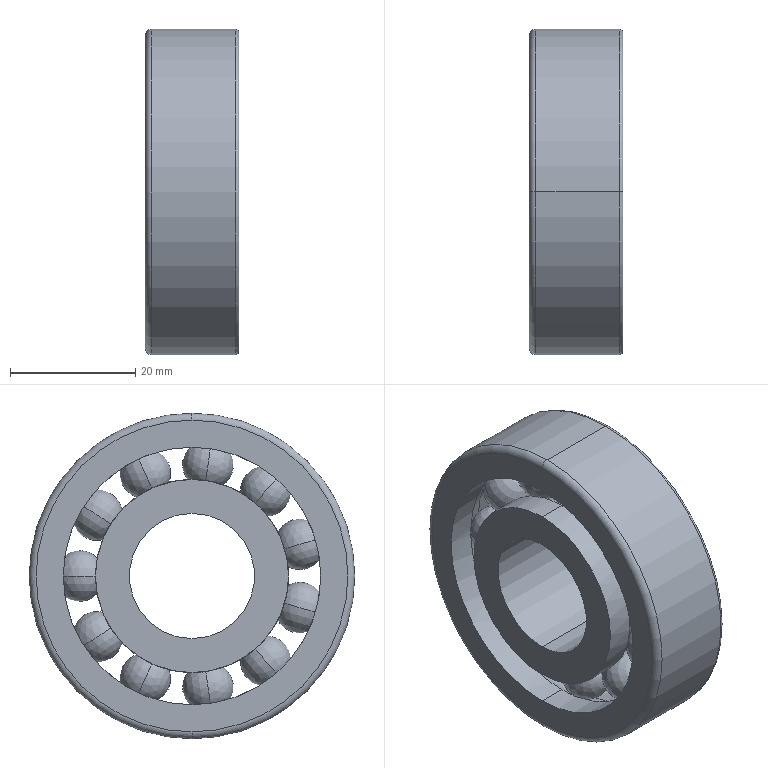Part | SolidWorks | features Revolution 3, Fillet 2, CirPattern 1 | 1 solid | 80 faces | box 15 x 52 x 52 mm | volume 18286 mm3 | torus 42 | sphere 22 | cylinder 10 | plane 4 | cone 2 | commonest cylinder face diameters 30.858 x4 20 x2 41.142 x2 52 x2